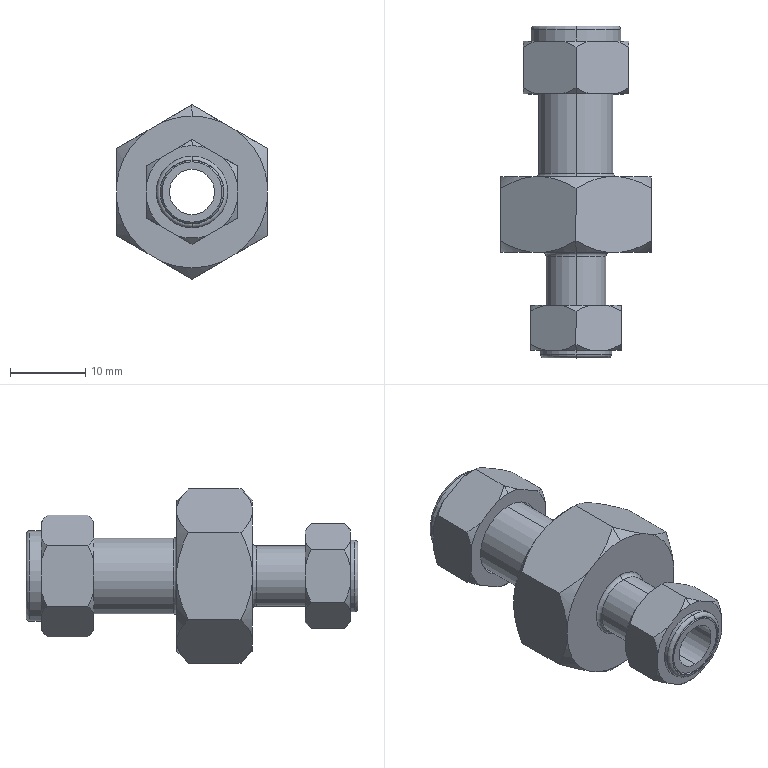Part | SolidWorks | features ICE 8, Fillet 3, Extrusion 1, RevCut 1 | 3 solids | 95 faces | box 20 x 44 x 23.094 mm | volume 5151 mm3 | cone 42 | plane 29 | cylinder 16 | torus 8 | commonest cylinder face diameters 8 x4 6 x2 8.4 x2 9.5 x2 10 x2 10.5 x2